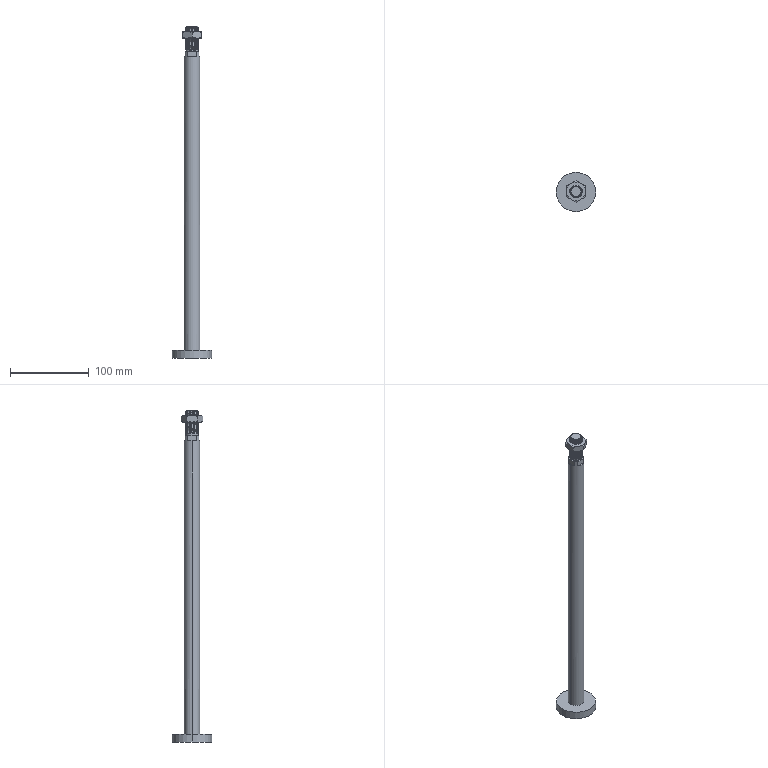Part | SolidWorks | features ICE 5, Revolution 3, RevCut 2, Chamfer 1, Helix 1, LPattern 1, MirrorPattern 1, SweepCut 1 | 1 solid | 78 faces | box 50 x 50 x 422.5 mm | volume 146980 mm3 | cylinder 37 | plane 23 | cone 14 | spline 4 | commonest cylinder face diameters 16 x31 14 x2 20 x2 50 x2